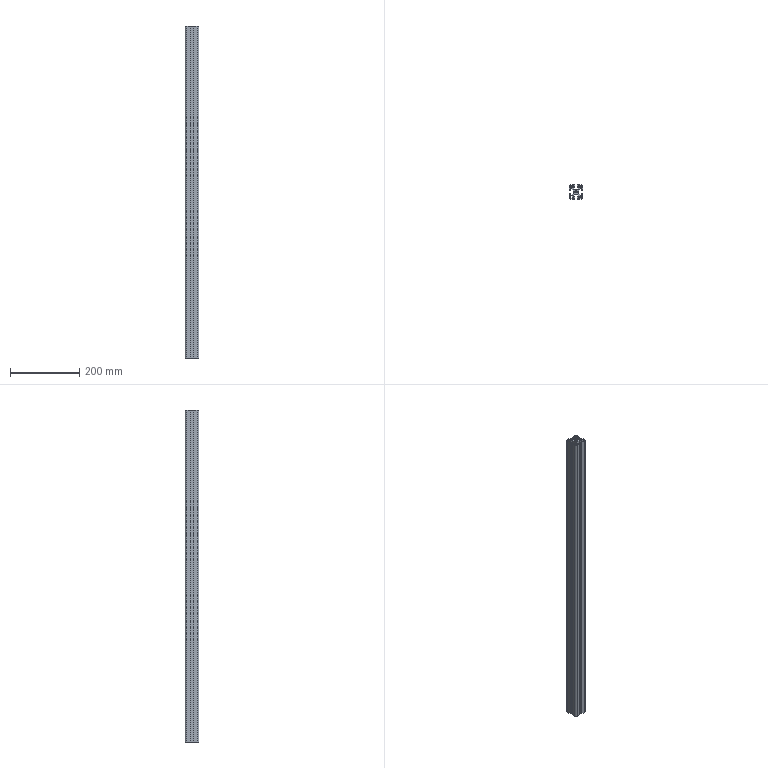Part | STEP file | 4040-960 | 1 solid | 88 faces | box 40 x 40 x 960 mm | volume 675789 mm3 | plane 78 | cylinder 10 | commonest cylinder face diameters 4 x4 10 x4 6.8 x2